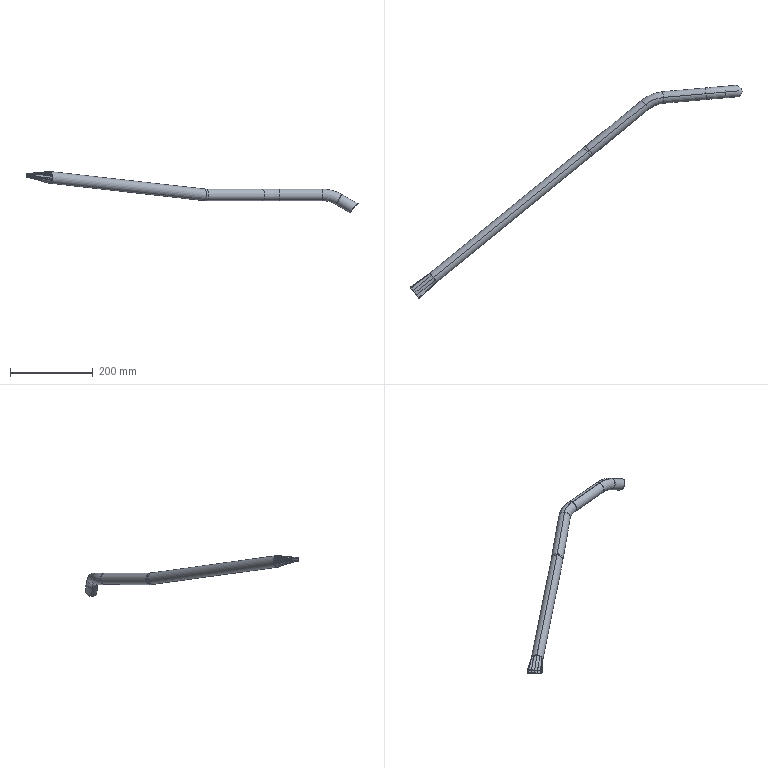Part | STEP file | PRT0001_68_3 | 1 solid | 103 faces | box 800.156 x 514.114 x 98.789 mm | volume 118663 mm3 | spline 71 | cylinder 18 | torus 12 | plane 2 | commonest cylinder face diameters 25 x8 28 x8 50 x1 2147 x1